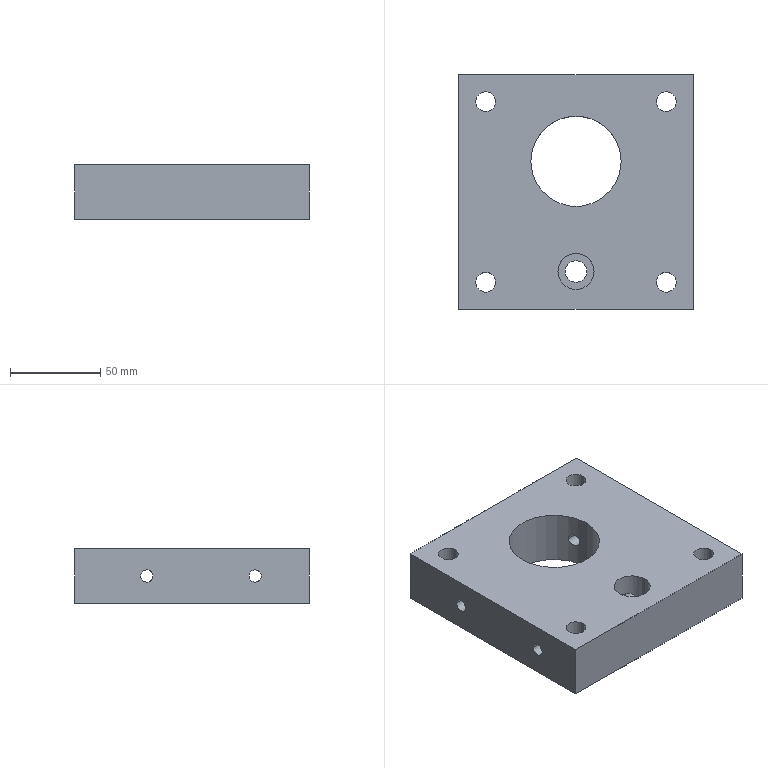Part | SolidWorks | features BaseBody 1 | 1 solid | 39 faces | box 130 x 130 x 30 mm | volume 407669 mm3 | cylinder 28 | plane 11 | commonest cylinder face diameters 20 x10 11 x8 6.8 x6 12 x2 50 x2